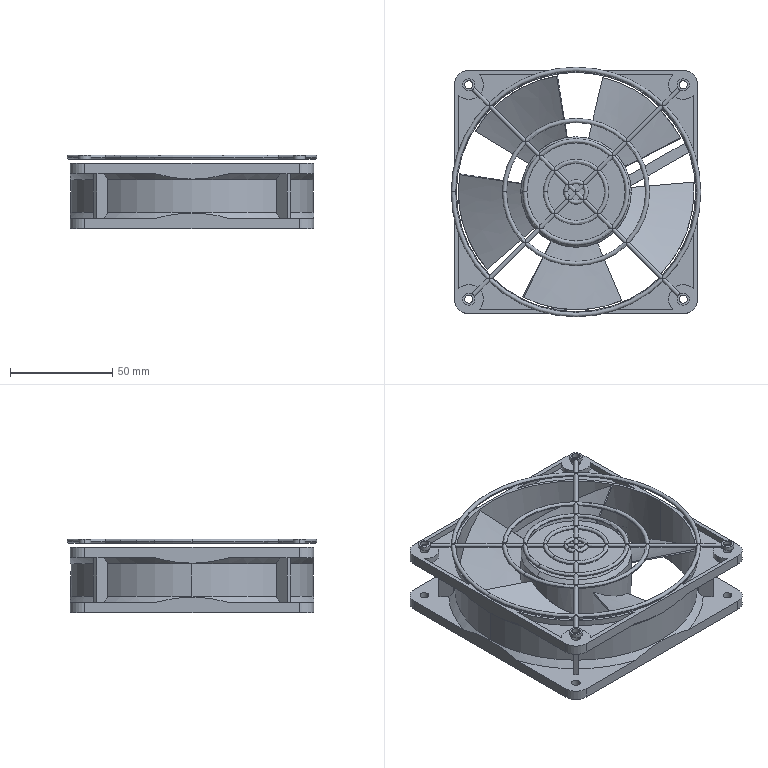Part | STEP file | 3 solids | 287 faces | box 122 x 122 x 36 mm | volume 116866 mm3 | cylinder 132 | plane 89 | torus 46 | spline 14 | cone 6 | commonest cylinder face diameters 2 x48 14.2 x20 4.3 x16 6 x12 119.559 x12 4 x8